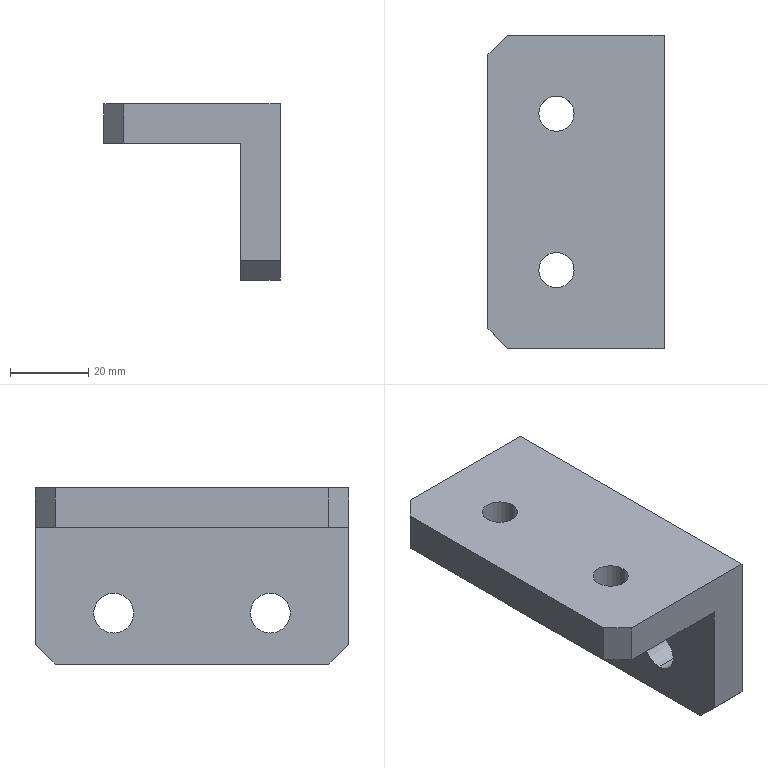Part | SolidWorks | features 3DProfileFeature 2, HoleWzd 2, Chamfer 1, Extrusion 1, LPattern 1 | 1 solid | 20 faces | box 45 x 80 x 45 mm | volume 60593 mm3 | plane 12 | cylinder 8 | commonest cylinder face diameters 9 x4 10.2 x4
STEP:
#1=CARTESIAN_POINT('',(22.5,20.,-14.6));
#2=VERTEX_POINT('',#1);
#3=CARTESIAN_POINT('',(22.5,20.,-4.4));
#4=VERTEX_POINT('',#3);
#5=CARTESIAN_POINT('',(22.5,20.,-9.5));
#6=DIRECTION('',(-1.,0.,0.));
#7=DIRECTION('',(0.,0.,1.));
#8=AXIS2_PLACEMENT_3D('',#5,#6,#7);
#9=CIRCLE('',#8,5.1);
#10=EDGE_CURVE('',#2,#4,#9,.T.);
#11=ORIENTED_EDGE('',*,*,#10,.F.);
#12=CARTESIAN_POINT('',(12.5,20.,-14.6));
#13=VERTEX_POINT('',#12);
#14=CARTESIAN_POINT('',(12.5,20.,-14.6));
#15=DIRECTION('',(-1.,0.,0.));
#16=VECTOR('',#15,1000.);
#17=LINE('',#14,#16);
#18=EDGE_CURVE('',#2,#13,#17,.T.);
#19=ORIENTED_EDGE('',*,*,#18,.T.);
#20=CARTESIAN_POINT('',(12.5,20.,-4.4));
#21=VERTEX_POINT('',#20);
#22=CARTESIAN_POINT('',(12.5,20.,-9.5));
#23=DIRECTION('',(-1.,0.,0.));
#24=DIRECTION('',(0.,0.,1.));
#25=AXIS2_PLACEMENT_3D('',#22,#23,#24);
#26=CIRCLE('',#25,5.1);
#27=EDGE_CURVE('',#13,#21,#26,.T.);
#28=ORIENTED_EDGE('',*,*,#27,.T.);
#29=CARTESIAN_POINT('',(12.5,20.,-4.4));
#30=DIRECTION('',(-1.,0.,0.));
#31=VECTOR('',#30,1000.);
#32=LINE('',#29,#31);
#33=EDGE_CURVE('',#4,#21,#32,.T.);
#34=ORIENTED_EDGE('',*,*,#33,.F.);
#35=EDGE_LOOP('',(#11,#19,#28,#34));
#36=FACE_OUTER_BOUND('',#35,.T.);
#37=CARTESIAN_POINT('',(12.5,20.,-9.5));
#38=DIRECTION('',(-1.,0.,0.));
#39=DIRECTION('',(0.,0.,1.));
#40=AXIS2_PLACEMENT_3D('',#37,#38,#39);
#41=CYLINDRICAL_SURFACE('',#40,5.1);
#42=ADVANCED_FACE('',(#36),#41,.F.);
#43=CARTESIAN_POINT('',(22.5,60.,-14.6));
#44=VERTEX_POINT('',#43);
#45=CARTESIAN_POINT('',(22.5,60.,-4.4));
#46=VERTEX_POINT('',#45);
#47=CARTESIAN_POINT('',(22.5,60.,-9.5));
#48=DIRECTION('',(-1.,0.,0.));
#49=DIRECTION('',(0.,0.,1.));
#50=AXIS2_PLACEMENT_3D('',#47,#48,#49);
#51=CIRCLE('',#50,5.1);
#52=EDGE_CURVE('',#44,#46,#51,.T.);
#53=ORIENTED_EDGE('',*,*,#52,.F.);
#54=CARTESIAN_POINT('',(12.5,60.,-14.6));
#55=VERTEX_POINT('',#54);
#56=CARTESIAN_POINT('',(12.5,60.,-14.6));
#57=DIRECTION('',(-1.,0.,0.));
#58=VECTOR('',#57,1000.);
#59=LINE('',#56,#58);
#60=EDGE_CURVE('',#44,#55,#59,.T.);
#61=ORIENTED_EDGE('',*,*,#60,.T.);
#62=CARTESIAN_POINT('',(12.5,60.,-4.4));
#63=VERTEX_POINT('',#62);
#64=CARTESIAN_POINT('',(12.5,60.,-9.5));
#65=DIRECTION('',(-1.,0.,0.));
#66=DIRECTION('',(0.,0.,1.));
#67=AXIS2_PLACEMENT_3D('',#64,#65,#66);
#68=CIRCLE('',#67,5.1);
#69=EDGE_CURVE('',#55,#63,#68,.T.);
#70=ORIENTED_EDGE('',*,*,#69,.T.);
#71=CARTESIAN_POINT('',(12.5,60.,-4.4));
#72=DIRECTION('',(-1.,0.,0.));
#73=VECTOR('',#72,1000.);
#74=LINE('',#71,#73);
#75=EDGE_CURVE('',#46,#63,#74,.T.);
#76=ORIENTED_EDGE('',*,*,#75,.F.);
#77=EDGE_LOOP('',(#53,#61,#70,#76));
#78=FACE_OUTER_BOUND('',#77,.T.);
#79=CARTESIAN_POINT('',(12.5,60.,-9.5));
#80=DIRECTION('',(-1.,0.,0.));
#81=DIRECTION('',(0.,0.,1.));
#82=AXIS2_PLACEMENT_3D('',#79,#80,#81);
#83=CYLINDRICAL_SURFACE('',#82,5.1);
#84=ADVANCED_FACE('',(#78),#83,.F.);
#85=CARTESIAN_POINT('',(-0.5,60.,22.5));
#86=VERTEX_POINT('',#85);
#87=CARTESIAN_POINT('',(-9.5,60.,22.5));
#88=VERTEX_POINT('',#87);
#89=CARTESIAN_POINT('',(-5.,60.,22.5));
#90=DIRECTION('',(0.,0.,-1.));
#91=DIRECTION('',(-1.,0.,0.));
#92=AXIS2_PLACEMENT_3D('',#89,#90,#91);
#93=CIRCLE('',#92,4.5);
#94=EDGE_CURVE('',#86,#88,#93,.T.);
#95=ORIENTED_EDGE('',*,*,#94,.F.);
#96=CARTESIAN_POINT('',(-0.5,60.,12.5));
#97=VERTEX_POINT('',#96);
#98=CARTESIAN_POINT('',(-0.5,60.,12.5));
#99=DIRECTION('',(0.,0.,-1.));
#100=VECTOR('',#99,1000.);
#101=LINE('',#98,#100);
#102=EDGE_CURVE('',#86,#97,#101,.T.);
#103=ORIENTED_EDGE('',*,*,#102,.T.);
#104=CARTESIAN_POINT('',(-9.5,60.,12.5));
#105=VERTEX_POINT('',#104);
#106=CARTESIAN_POINT('',(-5.,60.,12.5));
#107=DIRECTION('',(0.,0.,-1.));
#108=DIRECTION('',(-1.,0.,0.));
#109=AXIS2_PLACEMENT_3D('',#106,#107,#108);
#110=CIRCLE('',#109,4.5);
#111=EDGE_CURVE('',#97,#105,#110,.T.);
#112=ORIENTED_EDGE('',*,*,#111,.T.);
#113=CARTESIAN_POINT('',(-9.5,60.,12.5));
#114=DIRECTION('',(0.,0.,-1.));
#115=VECTOR('',#114,1000.);
#116=LINE('',#113,#115);
#117=EDGE_CURVE('',#88,#105,#116,.T.);
#118=ORIENTED_EDGE('',*,*,#117,.F.);
#119=EDGE_LOOP('',(#95,#103,#112,#118));
#120=FACE_OUTER_BOUND('',#119,.T.);
#121=CARTESIAN_POINT('',(-5.,60.,12.5));
#122=DIRECTION('',(0.,0.,-1.));
#123=DIRECTION('',(-1.,0.,0.));
#124=AXIS2_PLACEMENT_3D('',#121,#122,#123);
#125=CYLINDRICAL_SURFACE('',#124,4.5);
#126=ADVANCED_FACE('',(#120),#125,.F.);
#127=CARTESIAN_POINT('',(-0.5,20.,22.5));
#128=VERTEX_POINT('',#127);
#129=CARTESIAN_POINT('',(-9.5,20.,22.5));
#130=VERTEX_POINT('',#129);
#131=CARTESIAN_POINT('',(-5.,20.,22.5));
#132=DIRECTION('',(0.,0.,-1.));
#133=DIRECTION('',(-1.,0.,0.));
#134=AXIS2_PLACEMENT_3D('',#131,#132,#133);
#135=CIRCLE('',#134,4.5);
#136=EDGE_CURVE('',#128,#130,#135,.T.);
#137=ORIENTED_EDGE('',*,*,#136,.F.);
#138=CARTESIAN_POINT('',(-0.5,20.,12.5));
#139=VERTEX_POINT('',#138);
#140=CARTESIAN_POINT('',(-0.5,20.,12.5));
#141=DIRECTION('',(0.,0.,-1.));
#142=VECTOR('',#141,1000.);
#143=LINE('',#140,#142);
#144=EDGE_CURVE('',#128,#139,#143,.T.);
#145=ORIENTED_EDGE('',*,*,#144,.T.);
#146=CARTESIAN_POINT('',(-9.5,20.,12.5));
#147=VERTEX_POINT('',#146);
#148=CARTESIAN_POINT('',(-5.,20.,12.5));
#149=DIRECTION('',(0.,0.,-1.));
#150=DIRECTION('',(-1.,0.,0.));
#151=AXIS2_PLACEMENT_3D('',#148,#149,#150);
#152=CIRCLE('',#151,4.5);
#153=EDGE_CURVE('',#139,#147,#152,.T.);
#154=ORIENTED_EDGE('',*,*,#153,.T.);
#155=CARTESIAN_POINT('',(-9.5,20.,12.5));
#156=DIRECTION('',(0.,0.,-1.));
#157=VECTOR('',#156,1000.);
#158=LINE('',#155,#157);
#159=EDGE_CURVE('',#130,#147,#158,.T.);
#160=ORIENTED_EDGE('',*,*,#159,.F.);
#161=EDGE_LOOP('',(#137,#145,#154,#160));
#162=FACE_OUTER_BOUND('',#161,.T.);
#163=CARTESIAN_POINT('',(-5.,20.,12.5));
#164=DIRECTION('',(0.,0.,-1.));
#165=DIRECTION('',(-1.,0.,0.));
#166=AXIS2_PLACEMENT_3D('',#163,#164,#165);
#167=CYLINDRICAL_SURFACE('',#166,4.5);
#168=ADVANCED_FACE('',(#162),#167,.F.);
#169=CARTESIAN_POINT('',(22.5,20.,-9.5));
#170=DIRECTION('',(-1.,0.,0.));
#171=DIRECTION('',(0.,0.,1.));
#172=AXIS2_PLACEMENT_3D('',#169,#170,#171);
#173=CIRCLE('',#172,5.1);
#174=EDGE_CURVE('',#4,#2,#173,.T.);
#175=ORIENTED_EDGE('',*,*,#174,.T.);
#176=ORIENTED_EDGE('',*,*,#10,.T.);
#177=EDGE_LOOP('',(#175,#176));
#178=FACE_BOUND('',#177,.T.);
#179=CARTESIAN_POINT('',(22.5,60.,-9.5));
#180=DIRECTION('',(-1.,0.,0.));
#181=DIRECTION('',(0.,0.,1.));
#182=AXIS2_PLACEMENT_3D('',#179,#180,#181);
#183=CIRCLE('',#182,5.1);
#184=EDGE_CURVE('',#46,#44,#183,.T.);
#185=ORIENTED_EDGE('',*,*,#184,.T.);
#186=ORIENTED_EDGE('',*,*,#52,.T.);
#187=EDGE_LOOP('',(#185,#186));
#188=FACE_BOUND('',#187,.T.);
#189=CARTESIAN_POINT('',(22.5,75.,-22.5));
#190=VERTEX_POINT('',#189);
#191=CARTESIAN_POINT('',(22.5,5.,-22.5));
#192=VERTEX_POINT('',#191);
#193=CARTESIAN_POINT('',(22.5,80.,-22.5));
#194=DIRECTION('',(0.,-1.,0.));
#195=VECTOR('',#194,1000.);
#196=LINE('',#193,#195);
#197=EDGE_CURVE('',#190,#192,#196,.T.);
#198=ORIENTED_EDGE('',*,*,#197,.F.);
#199=CARTESIAN_POINT('',(22.5,80.,-17.5));
#200=VERTEX_POINT('',#199);
#201=CARTESIAN_POINT('',(22.5,80.,-17.5));
#202=DIRECTION('',(0.,0.7071,0.7071));
#203=VECTOR('',#202,1000.);
#204=LINE('',#201,#203);
#205=EDGE_CURVE('',#190,#200,#204,.T.);
#206=ORIENTED_EDGE('',*,*,#205,.T.);
#207=CARTESIAN_POINT('',(22.5,80.,22.5));
#208=VERTEX_POINT('',#207);
#209=CARTESIAN_POINT('',(22.5,80.,-22.5));
#210=DIRECTION('',(0.,0.,-1.));
#211=VECTOR('',#210,1000.);
#212=LINE('',#209,#211);
#213=EDGE_CURVE('',#208,#200,#212,.T.);
#214=ORIENTED_EDGE('',*,*,#213,.F.);
#215=CARTESIAN_POINT('',(22.5,0.,22.5));
#216=VERTEX_POINT('',#215);
#217=CARTESIAN_POINT('',(22.5,80.,22.5));
#218=DIRECTION('',(0.,-1.,0.));
#219=VECTOR('',#218,1000.);
#220=LINE('',#217,#219);
#221=EDGE_CURVE('',#208,#216,#220,.T.);
#222=ORIENTED_EDGE('',*,*,#221,.T.);
#223=CARTESIAN_POINT('',(22.5,0.,-17.5));
#224=VERTEX_POINT('',#223);
#225=CARTESIAN_POINT('',(22.5,0.,-22.5));
#226=DIRECTION('',(0.,0.,-1.));
#227=VECTOR('',#226,1000.);
#228=LINE('',#225,#227);
#229=EDGE_CURVE('',#216,#224,#228,.T.);
#230=ORIENTED_EDGE('',*,*,#229,.T.);
#231=CARTESIAN_POINT('',(22.5,5.,-22.5));
#232=DIRECTION('',(0.,0.7071,-0.7071));
#233=VECTOR('',#232,1000.);
#234=LINE('',#231,#233);
#235=EDGE_CURVE('',#224,#192,#234,.T.);
#236=ORIENTED_EDGE('',*,*,#235,.T.);
#237=EDGE_LOOP('',(#198,#206,#214,#222,#230,#236));
#238=FACE_OUTER_BOUND('',#237,.T.);
#239=CARTESIAN_POINT('',(22.5,80.,-22.5));
#240=DIRECTION('',(-1.,0.,0.));
#241=DIRECTION('',(0.,0.,1.));
#242=AXIS2_PLACEMENT_3D('',#239,#240,#241);
#243=PLANE('',#242);
#244=ADVANCED_FACE('',(#178,#188,#238),#243,.F.);
#245=CARTESIAN_POINT('',(12.5,75.,-22.5));
#246=VERTEX_POINT('',#245);
#247=CARTESIAN_POINT('',(12.5,5.,-22.5));
#248=VERTEX_POINT('',#247);
#249=CARTESIAN_POINT('',(12.5,80.,-22.5));
#250=DIRECTION('',(0.,-1.,0.));
#251=VECTOR('',#250,1000.);
#252=LINE('',#249,#251);
#253=EDGE_CURVE('',#246,#248,#252,.T.);
#254=ORIENTED_EDGE('',*,*,#253,.F.);
#255=CARTESIAN_POINT('',(22.5,75.,-22.5));
#256=DIRECTION('',(1.,0.,0.));
#257=VECTOR('',#256,1000.);
#258=LINE('',#255,#257);
#259=EDGE_CURVE('',#246,#190,#258,.T.);
#260=ORIENTED_EDGE('',*,*,#259,.T.);
#261=ORIENTED_EDGE('',*,*,#197,.T.);
#262=CARTESIAN_POINT('',(12.5,5.,-22.5));
#263=DIRECTION('',(-1.,0.,0.));
#264=VECTOR('',#263,1000.);
#265=LINE('',#262,#264);
#266=EDGE_CURVE('',#192,#248,#265,.T.);
#267=ORIENTED_EDGE('',*,*,#266,.T.);
#268=EDGE_LOOP('',(#254,#260,#261,#267));
#269=FACE_OUTER_BOUND('',#268,.T.);
#270=CARTESIAN_POINT('',(12.5,80.,-22.5));
#271=DIRECTION('',(0.,0.,1.));
#272=DIRECTION('',(1.,0.,0.));
#273=AXIS2_PLACEMENT_3D('',#270,#271,#272);
#274=PLANE('',#273);
#275=ADVANCED_FACE('',(#269),#274,.F.);
#276=CARTESIAN_POINT('',(12.5,20.,-9.5));
#277=DIRECTION('',(-1.,0.,0.));
#278=DIRECTION('',(0.,0.,1.));
#279=AXIS2_PLACEMENT_3D('',#276,#277,#278);
#280=CIRCLE('',#279,5.1);
#281=EDGE_CURVE('',#21,#13,#280,.T.);
#282=ORIENTED_EDGE('',*,*,#281,.F.);
#283=ORIENTED_EDGE('',*,*,#27,.F.);
#284=EDGE_LOOP('',(#282,#283));
#285=FACE_BOUND('',#284,.T.);
#286=CARTESIAN_POINT('',(12.5,60.,-9.5));
#287=DIRECTION('',(-1.,0.,0.));
#288=DIRECTION('',(0.,0.,1.));
#289=AXIS2_PLACEMENT_3D('',#286,#287,#288);
#290=CIRCLE('',#289,5.1);
#291=EDGE_CURVE('',#63,#55,#290,.T.);
#292=ORIENTED_EDGE('',*,*,#291,.F.);
#293=ORIENTED_EDGE('',*,*,#69,.F.);
#294=EDGE_LOOP('',(#292,#293));
#295=FACE_BOUND('',#294,.T.);
#296=CARTESIAN_POINT('',(12.5,80.,-17.5));
#297=VERTEX_POINT('',#296);
#298=CARTESIAN_POINT('',(12.5,80.,12.5));
#299=VERTEX_POINT('',#298);
#300=CARTESIAN_POINT('',(12.5,80.,-22.5));
#301=DIRECTION('',(0.,0.,1.));
#302=VECTOR('',#301,1000.);
#303=LINE('',#300,#302);
#304=EDGE_CURVE('',#297,#299,#303,.T.);
#305=ORIENTED_EDGE('',*,*,#304,.F.);
#306=CARTESIAN_POINT('',(12.5,80.,-17.5));
#307=DIRECTION('',(0.,-0.7071,-0.7071));
#308=VECTOR('',#307,1000.);
#309=LINE('',#306,#308);
#310=EDGE_CURVE('',#297,#246,#309,.T.);
#311=ORIENTED_EDGE('',*,*,#310,.T.);
#312=ORIENTED_EDGE('',*,*,#253,.T.);
#313=CARTESIAN_POINT('',(12.5,0.,-17.5));
#314=VERTEX_POINT('',#313);
#315=CARTESIAN_POINT('',(12.5,5.,-22.5));
#316=DIRECTION('',(0.,-0.7071,0.7071));
#317=VECTOR('',#316,1000.);
#318=LINE('',#315,#317);
#319=EDGE_CURVE('',#248,#314,#318,.T.);
#320=ORIENTED_EDGE('',*,*,#319,.T.);
#321=CARTESIAN_POINT('',(12.5,0.,12.5));
#322=VERTEX_POINT('',#321);
#323=CARTESIAN_POINT('',(12.5,0.,-22.5));
#324=DIRECTION('',(0.,0.,1.));
#325=VECTOR('',#324,1000.);
#326=LINE('',#323,#325);
#327=EDGE_CURVE('',#314,#322,#326,.T.);
#328=ORIENTED_EDGE('',*,*,#327,.T.);
#329=CARTESIAN_POINT('',(12.5,80.,12.5));
#330=DIRECTION('',(0.,-1.,0.));
#331=VECTOR('',#330,1000.);
#332=LINE('',#329,#331);
#333=EDGE_CURVE('',#299,#322,#332,.T.);
#334=ORIENTED_EDGE('',*,*,#333,.F.);
#335=EDGE_LOOP('',(#305,#311,#312,#320,#328,#334));
#336=FACE_OUTER_BOUND('',#335,.T.);
#337=CARTESIAN_POINT('',(12.5,80.,-22.5));
#338=DIRECTION('',(1.,0.,0.));
#339=DIRECTION('',(0.,0.,-1.));
#340=AXIS2_PLACEMENT_3D('',#337,#338,#339);
#341=PLANE('',#340);
#342=ADVANCED_FACE('',(#285,#295,#336),#341,.F.);
#343=CARTESIAN_POINT('',(-5.,60.,12.5));
#344=DIRECTION('',(0.,0.,-1.));
#345=DIRECTION('',(-1.,0.,0.));
#346=AXIS2_PLACEMENT_3D('',#343,#344,#345);
#347=CIRCLE('',#346,4.5);
#348=EDGE_CURVE('',#105,#97,#347,.T.);
#349=ORIENTED_EDGE('',*,*,#348,.F.);
#350=ORIENTED_EDGE('',*,*,#111,.F.);
#351=EDGE_LOOP('',(#349,#350));
#352=FACE_BOUND('',#351,.T.);
#353=CARTESIAN_POINT('',(-5.,20.,12.5));
#354=DIRECTION('',(0.,0.,-1.));
#355=DIRECTION('',(-1.,0.,0.));
#356=AXIS2_PLACEMENT_3D('',#353,#354,#355);
#357=CIRCLE('',#356,4.5);
#358=EDGE_CURVE('',#147,#139,#357,.T.);
#359=ORIENTED_EDGE('',*,*,#358,.F.);
#360=ORIENTED_EDGE('',*,*,#153,.F.);
#361=EDGE_LOOP('',(#359,#360));
#362=FACE_BOUND('',#361,.T.);
#363=CARTESIAN_POINT('',(-17.5,0.,12.5));
#364=VERTEX_POINT('',#363);
#365=CARTESIAN_POINT('',(-22.5,0.,12.5));
#366=DIRECTION('',(-1.,0.,0.));
#367=VECTOR('',#366,1000.);
#368=LINE('',#365,#367);
#369=EDGE_CURVE('',#322,#364,#368,.T.);
#370=ORIENTED_EDGE('',*,*,#369,.T.);
#371=CARTESIAN_POINT('',(-22.5,5.,12.5));
#372=VERTEX_POINT('',#371);
#373=CARTESIAN_POINT('',(-22.5,5.,12.5));
#374=DIRECTION('',(-0.7071,0.7071,0.));
#375=VECTOR('',#374,1000.);
#376=LINE('',#373,#375);
#377=EDGE_CURVE('',#364,#372,#376,.T.);
#378=ORIENTED_EDGE('',*,*,#377,.T.);
#379=CARTESIAN_POINT('',(-22.5,75.,12.5));
#380=VERTEX_POINT('',#379);
#381=CARTESIAN_POINT('',(-22.5,80.,12.5));
#382=DIRECTION('',(0.,-1.,0.));
#383=VECTOR('',#382,1000.);
#384=LINE('',#381,#383);
#385=EDGE_CURVE('',#380,#372,#384,.T.);
#386=ORIENTED_EDGE('',*,*,#385,.F.);
#387=CARTESIAN_POINT('',(-17.5,80.,12.5));
#388=VERTEX_POINT('',#387);
#389=CARTESIAN_POINT('',(-17.5,80.,12.5));
#390=DIRECTION('',(0.7071,0.7071,0.));
#391=VECTOR('',#390,1000.);
#392=LINE('',#389,#391);
#393=EDGE_CURVE('',#380,#388,#392,.T.);
#394=ORIENTED_EDGE('',*,*,#393,.T.);
#395=CARTESIAN_POINT('',(-22.5,80.,12.5));
#396=DIRECTION('',(-1.,0.,0.));
#397=VECTOR('',#396,1000.);
#398=LINE('',#395,#397);
#399=EDGE_CURVE('',#299,#388,#398,.T.);
#400=ORIENTED_EDGE('',*,*,#399,.F.);
#401=ORIENTED_EDGE('',*,*,#333,.T.);
#402=EDGE_LOOP('',(#370,#378,#386,#394,#400,#401));
#403=FACE_OUTER_BOUND('',#402,.T.);
#404=CARTESIAN_POINT('',(-22.5,80.,12.5));
#405=DIRECTION('',(0.,0.,1.));
#406=DIRECTION('',(1.,0.,0.));
#407=AXIS2_PLACEMENT_3D('',#404,#405,#406);
#408=PLANE('',#407);
#409=ADVANCED_FACE('',(#352,#362,#403),#408,.F.);
#410=ORIENTED_EDGE('',*,*,#385,.T.);
#411=CARTESIAN_POINT('',(-22.5,5.,22.5));
#412=VERTEX_POINT('',#411);
#413=CARTESIAN_POINT('',(-22.5,5.,12.5));
#414=DIRECTION('',(0.,0.,1.));
#415=VECTOR('',#414,1000.);
#416=LINE('',#413,#415);
#417=EDGE_CURVE('',#372,#412,#416,.T.);
#418=ORIENTED_EDGE('',*,*,#417,.T.);
#419=CARTESIAN_POINT('',(-22.5,75.,22.5));
#420=VERTEX_POINT('',#419);
#421=CARTESIAN_POINT('',(-22.5,80.,22.5));
#422=DIRECTION('',(0.,-1.,0.));
#423=VECTOR('',#422,1000.);
#424=LINE('',#421,#423);
#425=EDGE_CURVE('',#420,#412,#424,.T.);
#426=ORIENTED_EDGE('',*,*,#425,.F.);
#427=CARTESIAN_POINT('',(-22.5,75.,12.5));
#428=DIRECTION('',(0.,0.,-1.));
#429=VECTOR('',#428,1000.);
#430=LINE('',#427,#429);
#431=EDGE_CURVE('',#420,#380,#430,.T.);
#432=ORIENTED_EDGE('',*,*,#431,.T.);
#433=EDGE_LOOP('',(#410,#418,#426,#432));
#434=FACE_OUTER_BOUND('',#433,.T.);
#435=CARTESIAN_POINT('',(-22.5,80.,12.5));
#436=DIRECTION('',(1.,0.,0.));
#437=DIRECTION('',(0.,0.,-1.));
#438=AXIS2_PLACEMENT_3D('',#435,#436,#437);
#439=PLANE('',#438);
#440=ADVANCED_FACE('',(#434),#439,.F.);
#441=CARTESIAN_POINT('',(-5.,60.,22.5));
#442=DIRECTION('',(0.,0.,-1.));
#443=DIRECTION('',(-1.,0.,0.));
#444=AXIS2_PLACEMENT_3D('',#441,#442,#443);
#445=CIRCLE('',#444,4.5);
#446=EDGE_CURVE('',#88,#86,#445,.T.);
#447=ORIENTED_EDGE('',*,*,#446,.T.);
#448=ORIENTED_EDGE('',*,*,#94,.T.);
#449=EDGE_LOOP('',(#447,#448));
#450=FACE_BOUND('',#449,.T.);
#451=CARTESIAN_POINT('',(-5.,20.,22.5));
#452=DIRECTION('',(0.,0.,-1.));
#453=DIRECTION('',(-1.,0.,0.));
#454=AXIS2_PLACEMENT_3D('',#451,#452,#453);
#455=CIRCLE('',#454,4.5);
#456=EDGE_CURVE('',#130,#128,#455,.T.);
#457=ORIENTED_EDGE('',*,*,#456,.T.);
#458=ORIENTED_EDGE('',*,*,#136,.T.);
#459=EDGE_LOOP('',(#457,#458));
#460=FACE_BOUND('',#459,.T.);
#461=ORIENTED_EDGE('',*,*,#425,.T.);
#462=CARTESIAN_POINT('',(-17.5,0.,22.5));
#463=VERTEX_POINT('',#462);
#464=CARTESIAN_POINT('',(-22.5,5.,22.5));
#465=DIRECTION('',(0.7071,-0.7071,0.));
#466=VECTOR('',#465,1000.);
#467=LINE('',#464,#466);
#468=EDGE_CURVE('',#412,#463,#467,.T.);
#469=ORIENTED_EDGE('',*,*,#468,.T.);
#470=CARTESIAN_POINT('',(-22.5,0.,22.5));
#471=DIRECTION('',(1.,0.,0.));
#472=VECTOR('',#471,1000.);
#473=LINE('',#470,#472);
#474=EDGE_CURVE('',#463,#216,#473,.T.);
#475=ORIENTED_EDGE('',*,*,#474,.T.);
#476=ORIENTED_EDGE('',*,*,#221,.F.);
#477=CARTESIAN_POINT('',(-17.5,80.,22.5));
#478=VERTEX_POINT('',#477);
#479=CARTESIAN_POINT('',(-22.5,80.,22.5));
#480=DIRECTION('',(1.,0.,0.));
#481=VECTOR('',#480,1000.);
#482=LINE('',#479,#481);
#483=EDGE_CURVE('',#478,#208,#482,.T.);
#484=ORIENTED_EDGE('',*,*,#483,.F.);
#485=CARTESIAN_POINT('',(-17.5,80.,22.5));
#486=DIRECTION('',(-0.7071,-0.7071,0.));
#487=VECTOR('',#486,1000.);
#488=LINE('',#485,#487);
#489=EDGE_CURVE('',#478,#420,#488,.T.);
#490=ORIENTED_EDGE('',*,*,#489,.T.);
#491=EDGE_LOOP('',(#461,#469,#475,#476,#484,#490));
#492=FACE_OUTER_BOUND('',#491,.T.);
#493=CARTESIAN_POINT('',(-22.5,80.,22.5));
#494=DIRECTION('',(0.,0.,-1.));
#495=DIRECTION('',(-1.,0.,0.));
#496=AXIS2_PLACEMENT_3D('',#493,#494,#495);
#497=PLANE('',#496);
#498=ADVANCED_FACE('',(#450,#460,#492),#497,.F.);
#499=ORIENTED_EDGE('',*,*,#399,.T.);
#500=CARTESIAN_POINT('',(-17.5,80.,22.5));
#501=DIRECTION('',(0.,0.,1.));
#502=VECTOR('',#501,1000.);
#503=LINE('',#500,#502);
#504=EDGE_CURVE('',#388,#478,#503,.T.);
#505=ORIENTED_EDGE('',*,*,#504,.T.);
#506=ORIENTED_EDGE('',*,*,#483,.T.);
#507=ORIENTED_EDGE('',*,*,#213,.T.);
#508=CARTESIAN_POINT('',(12.5,80.,-17.5));
#509=DIRECTION('',(-1.,0.,0.));
#510=VECTOR('',#509,1000.);
#511=LINE('',#508,#510);
#512=EDGE_CURVE('',#200,#297,#511,.T.);
#513=ORIENTED_EDGE('',*,*,#512,.T.);
#514=ORIENTED_EDGE('',*,*,#304,.T.);
#515=EDGE_LOOP('',(#499,#505,#506,#507,#513,#514));
#516=FACE_OUTER_BOUND('',#515,.T.);
#517=CARTESIAN_POINT('',(0.,80.,0.));
#518=DIRECTION('',(0.,1.,0.));
#519=DIRECTION('',(0.,0.,1.));
#520=AXIS2_PLACEMENT_3D('',#517,#518,#519);
#521=PLANE('',#520);
#522=ADVANCED_FACE('',(#516),#521,.T.);
#523=ORIENTED_EDGE('',*,*,#474,.F.);
#524=CARTESIAN_POINT('',(-17.5,0.,0.));
#525=DIRECTION('',(0.,0.,-1.));
#526=VECTOR('',#525,1000.);
#527=LINE('',#524,#526);
#528=EDGE_CURVE('',#463,#364,#527,.T.);
#529=ORIENTED_EDGE('',*,*,#528,.T.);
#530=ORIENTED_EDGE('',*,*,#369,.F.);
#531=ORIENTED_EDGE('',*,*,#327,.F.);
#532=CARTESIAN_POINT('',(0.,0.,-17.5));
#533=DIRECTION('',(1.,0.,0.));
#534=VECTOR('',#533,1000.);
#535=LINE('',#532,#534);
#536=EDGE_CURVE('',#314,#224,#535,.T.);
#537=ORIENTED_EDGE('',*,*,#536,.T.);
#538=ORIENTED_EDGE('',*,*,#229,.F.);
#539=EDGE_LOOP('',(#523,#529,#530,#531,#537,#538));
#540=FACE_OUTER_BOUND('',#539,.T.);
#541=CARTESIAN_POINT('',(0.,0.,0.));
#542=DIRECTION('',(0.,1.,0.));
#543=DIRECTION('',(0.,0.,1.));
#544=AXIS2_PLACEMENT_3D('',#541,#542,#543);
#545=PLANE('',#544);
#546=ADVANCED_FACE('',(#540),#545,.F.);
#547=ORIENTED_EDGE('',*,*,#377,.F.);
#548=ORIENTED_EDGE('',*,*,#528,.F.);
#549=ORIENTED_EDGE('',*,*,#468,.F.);
#550=ORIENTED_EDGE('',*,*,#417,.F.);
#551=EDGE_LOOP('',(#547,#548,#549,#550));
#552=FACE_OUTER_BOUND('',#551,.T.);
#553=CARTESIAN_POINT('',(-22.5,5.,12.5));
#554=DIRECTION('',(0.7071,0.7071,0.));
#555=DIRECTION('',(0.,0.,1.));
#556=AXIS2_PLACEMENT_3D('',#553,#554,#555);
#557=PLANE('',#556);
#558=ADVANCED_FACE('',(#552),#557,.F.);
#559=ORIENTED_EDGE('',*,*,#393,.F.);
#560=ORIENTED_EDGE('',*,*,#431,.F.);
#561=ORIENTED_EDGE('',*,*,#489,.F.);
#562=ORIENTED_EDGE('',*,*,#504,.F.);
#563=EDGE_LOOP('',(#559,#560,#561,#562));
#564=FACE_OUTER_BOUND('',#563,.T.);
#565=CARTESIAN_POINT('',(-17.5,80.,0.));
#566=DIRECTION('',(-0.7071,0.7071,0.));
#567=DIRECTION('',(0.,0.,-1.));
#568=AXIS2_PLACEMENT_3D('',#565,#566,#567);
#569=PLANE('',#568);
#570=ADVANCED_FACE('',(#564),#569,.T.);
#571=ORIENTED_EDGE('',*,*,#205,.F.);
#572=ORIENTED_EDGE('',*,*,#259,.F.);
#573=ORIENTED_EDGE('',*,*,#310,.F.);
#574=ORIENTED_EDGE('',*,*,#512,.F.);
#575=EDGE_LOOP('',(#571,#572,#573,#574));
#576=FACE_OUTER_BOUND('',#575,.T.);
#577=CARTESIAN_POINT('',(0.,80.,-17.5));
#578=DIRECTION('',(0.,0.7071,-0.7071));
#579=DIRECTION('',(1.,0.,0.));
#580=AXIS2_PLACEMENT_3D('',#577,#578,#579);
#581=PLANE('',#580);
#582=ADVANCED_FACE('',(#576),#581,.T.);
#583=ORIENTED_EDGE('',*,*,#235,.F.);
#584=ORIENTED_EDGE('',*,*,#536,.F.);
#585=ORIENTED_EDGE('',*,*,#319,.F.);
#586=ORIENTED_EDGE('',*,*,#266,.F.);
#587=EDGE_LOOP('',(#583,#584,#585,#586));
#588=FACE_OUTER_BOUND('',#587,.T.);
#589=CARTESIAN_POINT('',(12.5,5.,-22.5));
#590=DIRECTION('',(0.,0.7071,0.7071));
#591=DIRECTION('',(-1.,0.,0.));
#592=AXIS2_PLACEMENT_3D('',#589,#590,#591);
#593=PLANE('',#592);
#594=ADVANCED_FACE('',(#588),#593,.F.);
#595=ORIENTED_EDGE('',*,*,#144,.F.);
#596=ORIENTED_EDGE('',*,*,#456,.F.);
#597=ORIENTED_EDGE('',*,*,#159,.T.);
#598=ORIENTED_EDGE('',*,*,#358,.T.);
#599=EDGE_LOOP('',(#595,#596,#597,#598));
#600=FACE_OUTER_BOUND('',#599,.T.);
#601=CARTESIAN_POINT('',(-5.,20.,12.5));
#602=DIRECTION('',(0.,0.,-1.));
#603=DIRECTION('',(-1.,0.,0.));
#604=AXIS2_PLACEMENT_3D('',#601,#602,#603);
#605=CYLINDRICAL_SURFACE('',#604,4.5);
#606=ADVANCED_FACE('',(#600),#605,.F.);
#607=ORIENTED_EDGE('',*,*,#102,.F.);
#608=ORIENTED_EDGE('',*,*,#446,.F.);
#609=ORIENTED_EDGE('',*,*,#117,.T.);
#610=ORIENTED_EDGE('',*,*,#348,.T.);
#611=EDGE_LOOP('',(#607,#608,#609,#610));
#612=FACE_OUTER_BOUND('',#611,.T.);
#613=CARTESIAN_POINT('',(-5.,60.,12.5));
#614=DIRECTION('',(0.,0.,-1.));
#615=DIRECTION('',(-1.,0.,0.));
#616=AXIS2_PLACEMENT_3D('',#613,#614,#615);
#617=CYLINDRICAL_SURFACE('',#616,4.5);
#618=ADVANCED_FACE('',(#612),#617,.F.);
#619=ORIENTED_EDGE('',*,*,#60,.F.);
#620=ORIENTED_EDGE('',*,*,#184,.F.);
#621=ORIENTED_EDGE('',*,*,#75,.T.);
#622=ORIENTED_EDGE('',*,*,#291,.T.);
#623=EDGE_LOOP('',(#619,#620,#621,#622));
#624=FACE_OUTER_BOUND('',#623,.T.);
#625=CARTESIAN_POINT('',(12.5,60.,-9.5));
#626=DIRECTION('',(-1.,0.,0.));
#627=DIRECTION('',(0.,0.,1.));
#628=AXIS2_PLACEMENT_3D('',#625,#626,#627);
#629=CYLINDRICAL_SURFACE('',#628,5.1);
#630=ADVANCED_FACE('',(#624),#629,.F.);
#631=ORIENTED_EDGE('',*,*,#18,.F.);
#632=ORIENTED_EDGE('',*,*,#174,.F.);
#633=ORIENTED_EDGE('',*,*,#33,.T.);
#634=ORIENTED_EDGE('',*,*,#281,.T.);
#635=EDGE_LOOP('',(#631,#632,#633,#634));
#636=FACE_OUTER_BOUND('',#635,.T.);
#637=CARTESIAN_POINT('',(12.5,20.,-9.5));
#638=DIRECTION('',(-1.,0.,0.));
#639=DIRECTION('',(0.,0.,1.));
#640=AXIS2_PLACEMENT_3D('',#637,#638,#639);
#641=CYLINDRICAL_SURFACE('',#640,5.1);
#642=ADVANCED_FACE('',(#636),#641,.F.);
#643=CLOSED_SHELL('',(#42,#84,#126,#168,#244,#275,#342,#409,#440,#498,#522,#546,#558,#570,#582,#594,#606,#618,#630,#642));
#644=MANIFOLD_SOLID_BREP('',#643);
#645=CARTESIAN_POINT('',(0.,0.,0.));
#646=DIRECTION('',(0.,0.,1.));
#647=DIRECTION('',(1.,0.,0.));
#648=AXIS2_PLACEMENT_3D('',#645,#646,#647);
#649=(LENGTH_UNIT()NAMED_UNIT(*)SI_UNIT(.MILLI.,.METRE.));
#650=UNCERTAINTY_MEASURE_WITH_UNIT(LENGTH_MEASURE(0.00001),#649,'','');
#651=(NAMED_UNIT(*)PLANE_ANGLE_UNIT()SI_UNIT($,.RADIAN.));
#652=(NAMED_UNIT(*)SI_UNIT($,.STERADIAN.)SOLID_ANGLE_UNIT());
#653=(GEOMETRIC_REPRESENTATION_CONTEXT(3)GLOBAL_UNCERTAINTY_ASSIGNED_CONTEXT((#650))GLOBAL_UNIT_ASSIGNED_CONTEXT((#649,#651,#652))REPRESENTATION_CONTEXT('',''));
#654=ADVANCED_BREP_SHAPE_REPRESENTATION('',(#644,#648),#653);